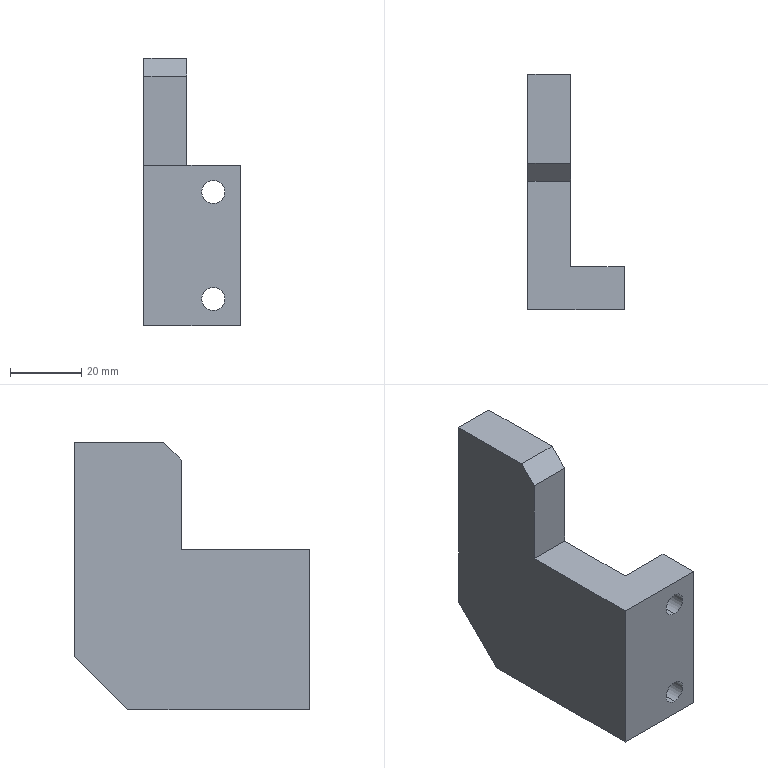Part | STEP file | material split support plate | 1 solid | 24 faces | box 27 x 66 x 75 mm | volume 51635 mm3 | plane 12 | cylinder 8 | cone 4 | commonest cylinder face diameters 5 x4 6.5 x4